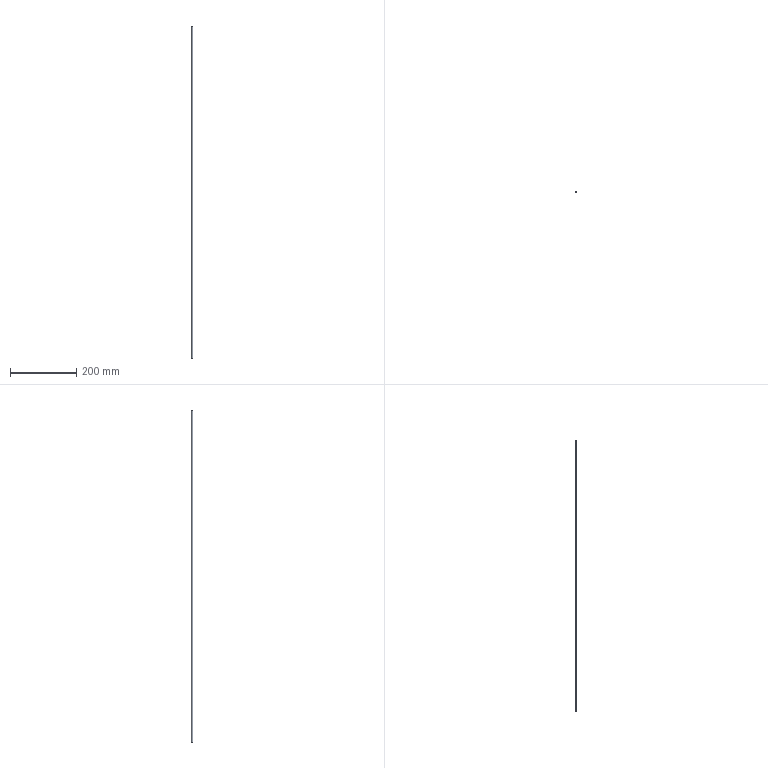Part | STEP file | P1 | 1 solid | 3 faces | box 4 x 4 x 1000 mm | volume 12566 mm3 | plane 2 | cylinder 1 | commonest cylinder face diameters 4 x1
STEP:
#1=CARTESIAN_POINT('',(0.,0.,0.));
#2=DIRECTION('',(0.,0.,1.));
#3=DIRECTION('',(1.,0.,0.));
#4=AXIS2_PLACEMENT_3D('',#1,#2,#3);
#5=CARTESIAN_POINT('',(2.,0.,1000.));
#6=VERTEX_POINT('',#5);
#7=CARTESIAN_POINT('',(0.,0.,1000.));
#8=DIRECTION('',(0.,0.,-1.));
#9=DIRECTION('',(-1.,0.,0.));
#10=AXIS2_PLACEMENT_3D('',#7,#8,#9);
#11=CIRCLE('',#10,2.);
#12=CARTESIAN_POINT('',(0.,0.,0.));
#13=DIRECTION('',(0.,0.,1.));
#14=DIRECTION('',(-1.,0.,0.));
#15=AXIS2_PLACEMENT_3D('',#12,#13,#14);
#16=CYLINDRICAL_SURFACE('',#15,2.);
#17=CARTESIAN_POINT('',(12.566,1000.));
#18=DIRECTION('',(-1.,0.));
#19=VECTOR('',#18,1.);
#20=LINE('',#17,#19);
#21=(GEOMETRIC_REPRESENTATION_CONTEXT(2)PARAMETRIC_REPRESENTATION_CONTEXT()REPRESENTATION_CONTEXT('',''));
#22=DEFINITIONAL_REPRESENTATION('',(#20),#21);
#23=PCURVE('',#16,#22);
#24=CARTESIAN_POINT('',(0.,0.,1000.));
#25=DIRECTION('',(0.,0.,1.));
#26=DIRECTION('',(1.,0.,0.));
#27=AXIS2_PLACEMENT_3D('',#24,#25,#26);
#28=PLANE('',#27);
#29=CARTESIAN_POINT('',(-2.,0.));
#30=CARTESIAN_POINT('',(-2.,3.464));
#31=CARTESIAN_POINT('',(1.,1.732));
#32=CARTESIAN_POINT('',(4.,0.));
#33=CARTESIAN_POINT('',(1.,-1.732));
#34=CARTESIAN_POINT('',(-2.,-3.464));
#35=CARTESIAN_POINT('',(-2.,0.));
#36=(BOUNDED_CURVE()B_SPLINE_CURVE(2,(#29,#30,#31,#32,#33,#34,#35),.UNSPECIFIED.,.T.,.F.)B_SPLINE_CURVE_WITH_KNOTS((1,2,2,2,2,1),(-2.094,0.,2.094,4.189,6.283,8.378),.UNSPECIFIED.)CURVE()GEOMETRIC_REPRESENTATION_ITEM()RATIONAL_B_SPLINE_CURVE((1.,0.5,1.,0.5,1.,0.5,1.))REPRESENTATION_ITEM(''));
#37=(GEOMETRIC_REPRESENTATION_CONTEXT(2)PARAMETRIC_REPRESENTATION_CONTEXT()REPRESENTATION_CONTEXT('',''));
#38=DEFINITIONAL_REPRESENTATION('',(#36),#37);
#39=PCURVE('',#28,#38);
#40=SURFACE_CURVE('',#11,(#23,#39),.PCURVE_S1.);
#41=EDGE_CURVE('',#6,#6,#40,.T.);
#42=ORIENTED_EDGE('',*,*,#41,.T.);
#43=CARTESIAN_POINT('',(2.,0.,0.));
#44=VERTEX_POINT('',#43);
#45=CARTESIAN_POINT('',(2.,0.,0.));
#46=CARTESIAN_POINT('',(2.,0.,1000.));
#47=B_SPLINE_CURVE_WITH_KNOTS('',1,(#45,#46),.UNSPECIFIED.,.F.,.F.,(2,2),(0.,1000.),.PIECEWISE_BEZIER_KNOTS.);
#48=CARTESIAN_POINT('',(3.142,0.));
#49=DIRECTION('',(0.,1.));
#50=VECTOR('',#49,1.);
#51=LINE('',#48,#50);
#52=(GEOMETRIC_REPRESENTATION_CONTEXT(2)PARAMETRIC_REPRESENTATION_CONTEXT()REPRESENTATION_CONTEXT('',''));
#53=DEFINITIONAL_REPRESENTATION('',(#51),#52);
#54=PCURVE('',#16,#53);
#55=CARTESIAN_POINT('',(9.425,0.));
#56=DIRECTION('',(0.,1.));
#57=VECTOR('',#56,1.);
#58=LINE('',#55,#57);
#59=(GEOMETRIC_REPRESENTATION_CONTEXT(2)PARAMETRIC_REPRESENTATION_CONTEXT()REPRESENTATION_CONTEXT('',''));
#60=DEFINITIONAL_REPRESENTATION('',(#58),#59);
#61=PCURVE('',#16,#60);
#62=SEAM_CURVE('',#47,(#54,#61),.PCURVE_S1.);
#63=EDGE_CURVE('',#44,#6,#62,.T.);
#64=ORIENTED_EDGE('',*,*,#63,.F.);
#65=CARTESIAN_POINT('',(0.,0.,0.));
#66=DIRECTION('',(0.,0.,-1.));
#67=DIRECTION('',(-1.,0.,0.));
#68=AXIS2_PLACEMENT_3D('',#65,#66,#67);
#69=CIRCLE('',#68,2.);
#70=CARTESIAN_POINT('',(12.566,0.));
#71=DIRECTION('',(-1.,0.));
#72=VECTOR('',#71,1.);
#73=LINE('',#70,#72);
#74=(GEOMETRIC_REPRESENTATION_CONTEXT(2)PARAMETRIC_REPRESENTATION_CONTEXT()REPRESENTATION_CONTEXT('',''));
#75=DEFINITIONAL_REPRESENTATION('',(#73),#74);
#76=PCURVE('',#16,#75);
#77=CARTESIAN_POINT('',(0.,0.,0.));
#78=DIRECTION('',(0.,0.,1.));
#79=DIRECTION('',(1.,0.,0.));
#80=AXIS2_PLACEMENT_3D('',#77,#78,#79);
#81=PLANE('',#80);
#82=CARTESIAN_POINT('',(-2.,0.));
#83=CARTESIAN_POINT('',(-2.,3.464));
#84=CARTESIAN_POINT('',(1.,1.732));
#85=CARTESIAN_POINT('',(4.,0.));
#86=CARTESIAN_POINT('',(1.,-1.732));
#87=CARTESIAN_POINT('',(-2.,-3.464));
#88=CARTESIAN_POINT('',(-2.,0.));
#89=(BOUNDED_CURVE()B_SPLINE_CURVE(2,(#82,#83,#84,#85,#86,#87,#88),.UNSPECIFIED.,.T.,.F.)B_SPLINE_CURVE_WITH_KNOTS((1,2,2,2,2,1),(-2.094,0.,2.094,4.189,6.283,8.378),.UNSPECIFIED.)CURVE()GEOMETRIC_REPRESENTATION_ITEM()RATIONAL_B_SPLINE_CURVE((1.,0.5,1.,0.5,1.,0.5,1.))REPRESENTATION_ITEM(''));
#90=(GEOMETRIC_REPRESENTATION_CONTEXT(2)PARAMETRIC_REPRESENTATION_CONTEXT()REPRESENTATION_CONTEXT('',''));
#91=DEFINITIONAL_REPRESENTATION('',(#89),#90);
#92=PCURVE('',#81,#91);
#93=SURFACE_CURVE('',#69,(#76,#92),.PCURVE_S1.);
#94=EDGE_CURVE('',#44,#44,#93,.T.);
#95=ORIENTED_EDGE('',*,*,#94,.F.);
#96=ORIENTED_EDGE('',*,*,#63,.T.);
#97=EDGE_LOOP('',(#42,#64,#95,#96));
#98=FACE_BOUND('',#97,.T.);
#99=ADVANCED_FACE('',(#98),#16,.T.);
#100=ORIENTED_EDGE('',*,*,#94,.T.);
#101=EDGE_LOOP('',(#100));
#102=FACE_BOUND('',#101,.T.);
#103=ADVANCED_FACE('',(#102),#81,.F.);
#104=ORIENTED_EDGE('',*,*,#41,.F.);
#105=EDGE_LOOP('',(#104));
#106=FACE_BOUND('',#105,.T.);
#107=ADVANCED_FACE('',(#106),#28,.T.);
#108=CLOSED_SHELL('',(#99,#103,#107));
#109=MANIFOLD_SOLID_BREP('',#108);
#110=(LENGTH_UNIT()NAMED_UNIT(*)SI_UNIT(.MILLI.,.METRE.));
#111=UNCERTAINTY_MEASURE_WITH_UNIT(LENGTH_MEASURE(0.00001),#110,'','');
#112=(NAMED_UNIT(*)PLANE_ANGLE_UNIT()SI_UNIT($,.RADIAN.));
#113=(NAMED_UNIT(*)SI_UNIT($,.STERADIAN.)SOLID_ANGLE_UNIT());
#114=(GEOMETRIC_REPRESENTATION_CONTEXT(3)GLOBAL_UNCERTAINTY_ASSIGNED_CONTEXT((#111))GLOBAL_UNIT_ASSIGNED_CONTEXT((#110,#112,#113))REPRESENTATION_CONTEXT('',''));
#115=ADVANCED_BREP_SHAPE_REPRESENTATION('',(#4,#109),#114);